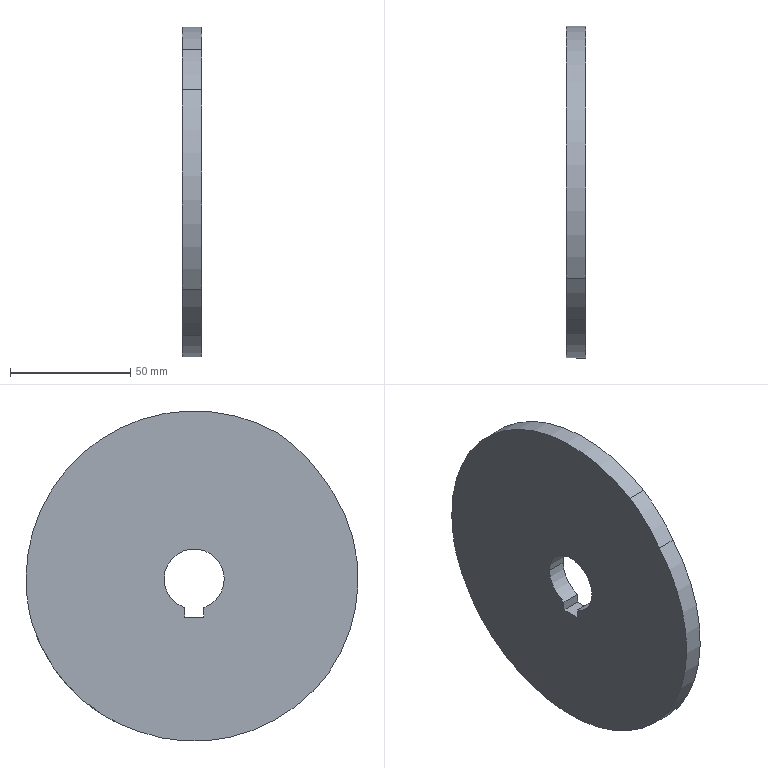Part | NX | 1 solid | 15 faces | box 8 x 138.01 x 137.3 mm | volume 114801 mm3 | cylinder 9 | plane 5 | spline 1 | commonest cylinder face diameters 25 x3 139.8 x2 134.8 x1 135.471 x1 136.22 x1 137.835 x1
STEP:
#1=CARTESIAN_POINT('',(-4.,67.518,-18.091));
#2=VERTEX_POINT('',#1);
#3=CARTESIAN_POINT('',(-4.,69.9,0.));
#4=VERTEX_POINT('',#3);
#5=CARTESIAN_POINT('',(-4.,0.,0.));
#6=DIRECTION('',(1.,0.,0.));
#7=DIRECTION('',(0.,1.,0.));
#8=AXIS2_PLACEMENT_3D('',#5,#6,#7);
#9=CIRCLE('',#8,69.9);
#10=EDGE_CURVE('',#2,#4,#9,.T.);
#11=ORIENTED_EDGE('',*,*,#10,.F.);
#12=CARTESIAN_POINT('',(-4.,23.052,-63.335));
#13=VERTEX_POINT('',#12);
#14=CARTESIAN_POINT('',(-4.,67.518,-18.091));
#15=CARTESIAN_POINT('',(-4.,64.222,-28.782));
#16=CARTESIAN_POINT('',(-4.,52.439,-48.353));
#17=CARTESIAN_POINT('',(-4.,33.356,-60.029));
#18=CARTESIAN_POINT('',(-4.,23.052,-63.335));
#19=B_SPLINE_CURVE_WITH_KNOTS('',3,(#14,#15,#16,#17,#18),.UNSPECIFIED.,.F.,.F.,(4,1,4),(0.,0.5,1.),.UNSPECIFIED.);
#20=EDGE_CURVE('',#13,#2,#19,.F.);
#21=ORIENTED_EDGE('',*,*,#20,.F.);
#22=CARTESIAN_POINT('',(-4.,-33.701,-58.37));
#23=VERTEX_POINT('',#22);
#24=CARTESIAN_POINT('',(-4.,0.,0.));
#25=DIRECTION('',(1.,0.,0.));
#26=DIRECTION('',(0.,-0.5001,-0.866));
#27=AXIS2_PLACEMENT_3D('',#24,#25,#26);
#28=CIRCLE('',#27,67.4);
#29=EDGE_CURVE('',#23,#13,#28,.T.);
#30=ORIENTED_EDGE('',*,*,#29,.F.);
#31=CARTESIAN_POINT('',(-4.,-55.792,-39.066));
#32=VERTEX_POINT('',#31);
#33=CARTESIAN_POINT('',(-4.,-1.234,1.077));
#34=DIRECTION('',(1.,0.,0.));
#35=DIRECTION('',(0.,-0.8055,-0.5926));
#36=AXIS2_PLACEMENT_3D('',#33,#34,#35);
#37=CIRCLE('',#36,67.736);
#38=EDGE_CURVE('',#32,#23,#37,.T.);
#39=ORIENTED_EDGE('',*,*,#38,.F.);
#40=CARTESIAN_POINT('',(-4.,-52.176,43.781));
#41=VERTEX_POINT('',#40);
#42=CARTESIAN_POINT('',(-4.,0.,0.));
#43=DIRECTION('',(1.,0.,0.));
#44=DIRECTION('',(0.,-0.766,0.6428));
#45=AXIS2_PLACEMENT_3D('',#42,#43,#44);
#46=CIRCLE('',#45,68.11);
#47=EDGE_CURVE('',#41,#32,#46,.T.);
#48=ORIENTED_EDGE('',*,*,#47,.F.);
#49=CARTESIAN_POINT('',(-4.,-34.947,60.538));
#50=VERTEX_POINT('',#49);
#51=CARTESIAN_POINT('',(-4.,3.752,3.512));
#52=DIRECTION('',(1.,0.,0.));
#53=DIRECTION('',(0.,-0.5615,0.8275));
#54=AXIS2_PLACEMENT_3D('',#51,#52,#53);
#55=CIRCLE('',#54,68.917);
#56=EDGE_CURVE('',#50,#41,#55,.T.);
#57=ORIENTED_EDGE('',*,*,#56,.F.);
#58=CARTESIAN_POINT('',(-4.,0.,0.));
#59=DIRECTION('',(1.,0.,0.));
#60=DIRECTION('',(0.,1.,0.));
#61=AXIS2_PLACEMENT_3D('',#58,#59,#60);
#62=CIRCLE('',#61,69.9);
#63=EDGE_CURVE('',#4,#50,#62,.T.);
#64=ORIENTED_EDGE('',*,*,#63,.F.);
#65=EDGE_LOOP('',(#11,#21,#30,#39,#48,#57,#64));
#66=FACE_BOUND('',#65,.T.);
#67=CARTESIAN_POINT('',(-4.,-4.,-11.843));
#68=VERTEX_POINT('',#67);
#69=CARTESIAN_POINT('',(-4.,-12.5,0.));
#70=VERTEX_POINT('',#69);
#71=CARTESIAN_POINT('',(-4.,0.,0.));
#72=DIRECTION('',(-1.,0.,0.));
#73=DIRECTION('',(0.,1.,0.));
#74=AXIS2_PLACEMENT_3D('',#71,#72,#73);
#75=CIRCLE('',#74,12.5);
#76=EDGE_CURVE('',#68,#70,#75,.T.);
#77=ORIENTED_EDGE('',*,*,#76,.F.);
#78=CARTESIAN_POINT('',(-4.,-4.,-15.8));
#79=VERTEX_POINT('',#78);
#80=CARTESIAN_POINT('',(-4.,-4.,-11.843));
#81=DIRECTION('',(0.,0.,-1.));
#82=VECTOR('',#81,1000.);
#83=LINE('',#80,#82);
#84=EDGE_CURVE('',#68,#79,#83,.T.);
#85=ORIENTED_EDGE('',*,*,#84,.T.);
#86=CARTESIAN_POINT('',(-4.,4.,-15.8));
#87=VERTEX_POINT('',#86);
#88=CARTESIAN_POINT('',(-4.,-4.,-15.8));
#89=DIRECTION('',(0.,1.,0.));
#90=VECTOR('',#89,1000.);
#91=LINE('',#88,#90);
#92=EDGE_CURVE('',#79,#87,#91,.T.);
#93=ORIENTED_EDGE('',*,*,#92,.T.);
#94=CARTESIAN_POINT('',(-4.,4.,-11.843));
#95=VERTEX_POINT('',#94);
#96=CARTESIAN_POINT('',(-4.,4.,-15.8));
#97=DIRECTION('',(0.,0.,1.));
#98=VECTOR('',#97,1000.);
#99=LINE('',#96,#98);
#100=EDGE_CURVE('',#87,#95,#99,.T.);
#101=ORIENTED_EDGE('',*,*,#100,.T.);
#102=CARTESIAN_POINT('',(-4.,12.5,0.));
#103=VERTEX_POINT('',#102);
#104=CARTESIAN_POINT('',(-4.,0.,0.));
#105=DIRECTION('',(-1.,0.,0.));
#106=DIRECTION('',(0.,1.,0.));
#107=AXIS2_PLACEMENT_3D('',#104,#105,#106);
#108=CIRCLE('',#107,12.5);
#109=EDGE_CURVE('',#103,#95,#108,.T.);
#110=ORIENTED_EDGE('',*,*,#109,.F.);
#111=CARTESIAN_POINT('',(-4.,0.,0.));
#112=DIRECTION('',(-1.,0.,0.));
#113=DIRECTION('',(0.,1.,0.));
#114=AXIS2_PLACEMENT_3D('',#111,#112,#113);
#115=CIRCLE('',#114,12.5);
#116=EDGE_CURVE('',#70,#103,#115,.T.);
#117=ORIENTED_EDGE('',*,*,#116,.F.);
#118=EDGE_LOOP('',(#77,#85,#93,#101,#110,#117));
#119=FACE_BOUND('',#118,.T.);
#120=CARTESIAN_POINT('',(-4.,0.,0.));
#121=DIRECTION('',(1.,0.,0.));
#122=DIRECTION('',(0.,1.,0.));
#123=AXIS2_PLACEMENT_3D('',#120,#121,#122);
#124=PLANE('',#123);
#125=ADVANCED_FACE('',(#66,#119),#124,.F.);
#126=CARTESIAN_POINT('',(4.,69.9,0.));
#127=VERTEX_POINT('',#126);
#128=CARTESIAN_POINT('',(4.,69.9,0.));
#129=DIRECTION('',(-1.,0.,0.));
#130=VECTOR('',#129,1000.);
#131=LINE('',#128,#130);
#132=EDGE_CURVE('',#127,#4,#131,.T.);
#133=ORIENTED_EDGE('',*,*,#132,.F.);
#134=CARTESIAN_POINT('',(4.,67.518,-18.091));
#135=VERTEX_POINT('',#134);
#136=CARTESIAN_POINT('',(4.,0.,0.));
#137=DIRECTION('',(-1.,0.,0.));
#138=DIRECTION('',(0.,-0.4999,0.8661));
#139=AXIS2_PLACEMENT_3D('',#136,#137,#138);
#140=CIRCLE('',#139,69.9);
#141=EDGE_CURVE('',#127,#135,#140,.T.);
#142=ORIENTED_EDGE('',*,*,#141,.T.);
#143=CARTESIAN_POINT('',(4.,67.518,-18.091));
#144=CARTESIAN_POINT('',(1.333,67.518,-18.091));
#145=CARTESIAN_POINT('',(-1.333,67.518,-18.091));
#146=CARTESIAN_POINT('',(-4.,67.518,-18.091));
#147=B_SPLINE_CURVE_WITH_KNOTS('',3,(#143,#144,#145,#146),.UNSPECIFIED.,.F.,.F.,(4,4),(0.,1.),.UNSPECIFIED.);
#148=EDGE_CURVE('',#135,#2,#147,.T.);
#149=ORIENTED_EDGE('',*,*,#148,.T.);
#150=ORIENTED_EDGE('',*,*,#10,.T.);
#151=EDGE_LOOP('',(#133,#142,#149,#150));
#152=FACE_BOUND('',#151,.T.);
#153=CARTESIAN_POINT('',(4.,0.,0.));
#154=DIRECTION('',(-1.,0.,0.));
#155=DIRECTION('',(0.,1.,0.));
#156=AXIS2_PLACEMENT_3D('',#153,#154,#155);
#157=CYLINDRICAL_SURFACE('',#156,69.9);
#158=ADVANCED_FACE('',(#152),#157,.T.);
#159=CARTESIAN_POINT('',(4.,-34.947,60.538));
#160=VERTEX_POINT('',#159);
#161=CARTESIAN_POINT('',(4.,0.,0.));
#162=DIRECTION('',(-1.,0.,0.));
#163=DIRECTION('',(0.,-0.4999,0.8661));
#164=AXIS2_PLACEMENT_3D('',#161,#162,#163);
#165=CIRCLE('',#164,69.9);
#166=EDGE_CURVE('',#160,#127,#165,.T.);
#167=ORIENTED_EDGE('',*,*,#166,.F.);
#168=CARTESIAN_POINT('',(4.,-52.176,43.781));
#169=VERTEX_POINT('',#168);
#170=CARTESIAN_POINT('',(4.,3.752,3.512));
#171=DIRECTION('',(-1.,0.,0.));
#172=DIRECTION('',(0.,-0.8115,0.5843));
#173=AXIS2_PLACEMENT_3D('',#170,#171,#172);
#174=CIRCLE('',#173,68.917);
#175=EDGE_CURVE('',#169,#160,#174,.T.);
#176=ORIENTED_EDGE('',*,*,#175,.F.);
#177=CARTESIAN_POINT('',(4.,-55.792,-39.066));
#178=VERTEX_POINT('',#177);
#179=CARTESIAN_POINT('',(4.,0.,0.));
#180=DIRECTION('',(-1.,0.,0.));
#181=DIRECTION('',(0.,-0.8192,-0.5735));
#182=AXIS2_PLACEMENT_3D('',#179,#180,#181);
#183=CIRCLE('',#182,68.11);
#184=EDGE_CURVE('',#178,#169,#183,.T.);
#185=ORIENTED_EDGE('',*,*,#184,.F.);
#186=CARTESIAN_POINT('',(4.,-33.701,-58.37));
#187=VERTEX_POINT('',#186);
#188=CARTESIAN_POINT('',(4.,-1.234,1.077));
#189=DIRECTION('',(-1.,0.,0.));
#190=DIRECTION('',(0.,-0.4794,-0.8776));
#191=AXIS2_PLACEMENT_3D('',#188,#189,#190);
#192=CIRCLE('',#191,67.736);
#193=EDGE_CURVE('',#187,#178,#192,.T.);
#194=ORIENTED_EDGE('',*,*,#193,.F.);
#195=CARTESIAN_POINT('',(4.,23.052,-63.335));
#196=VERTEX_POINT('',#195);
#197=CARTESIAN_POINT('',(4.,0.,0.));
#198=DIRECTION('',(-1.,0.,0.));
#199=DIRECTION('',(0.,0.342,-0.9397));
#200=AXIS2_PLACEMENT_3D('',#197,#198,#199);
#201=CIRCLE('',#200,67.4);
#202=EDGE_CURVE('',#196,#187,#201,.T.);
#203=ORIENTED_EDGE('',*,*,#202,.F.);
#204=CARTESIAN_POINT('',(4.,23.052,-63.335));
#205=CARTESIAN_POINT('',(4.,33.355,-60.03));
#206=CARTESIAN_POINT('',(4.,52.44,-48.352));
#207=CARTESIAN_POINT('',(4.,64.222,-28.783));
#208=CARTESIAN_POINT('',(4.,67.518,-18.091));
#209=B_SPLINE_CURVE_WITH_KNOTS('',3,(#204,#205,#206,#207,#208),.UNSPECIFIED.,.F.,.F.,(4,1,4),(0.,0.5,1.),.UNSPECIFIED.);
#210=EDGE_CURVE('',#135,#196,#209,.F.);
#211=ORIENTED_EDGE('',*,*,#210,.F.);
#212=ORIENTED_EDGE('',*,*,#141,.F.);
#213=EDGE_LOOP('',(#167,#176,#185,#194,#203,#211,#212));
#214=FACE_BOUND('',#213,.T.);
#215=CARTESIAN_POINT('',(4.,4.,-11.843));
#216=VERTEX_POINT('',#215);
#217=CARTESIAN_POINT('',(4.,12.5,0.));
#218=VERTEX_POINT('',#217);
#219=CARTESIAN_POINT('',(4.,0.,0.));
#220=DIRECTION('',(1.,0.,0.));
#221=DIRECTION('',(0.,-1.,0.));
#222=AXIS2_PLACEMENT_3D('',#219,#220,#221);
#223=CIRCLE('',#222,12.5);
#224=EDGE_CURVE('',#216,#218,#223,.T.);
#225=ORIENTED_EDGE('',*,*,#224,.F.);
#226=CARTESIAN_POINT('',(4.,4.,-15.8));
#227=VERTEX_POINT('',#226);
#228=CARTESIAN_POINT('',(4.,4.,-15.8));
#229=DIRECTION('',(0.,0.,1.));
#230=VECTOR('',#229,1000.);
#231=LINE('',#228,#230);
#232=EDGE_CURVE('',#227,#216,#231,.T.);
#233=ORIENTED_EDGE('',*,*,#232,.F.);
#234=CARTESIAN_POINT('',(4.,-4.,-15.8));
#235=VERTEX_POINT('',#234);
#236=CARTESIAN_POINT('',(4.,-4.,-15.8));
#237=DIRECTION('',(0.,1.,0.));
#238=VECTOR('',#237,1000.);
#239=LINE('',#236,#238);
#240=EDGE_CURVE('',#235,#227,#239,.T.);
#241=ORIENTED_EDGE('',*,*,#240,.F.);
#242=CARTESIAN_POINT('',(4.,-4.,-11.843));
#243=VERTEX_POINT('',#242);
#244=CARTESIAN_POINT('',(4.,-4.,-11.843));
#245=DIRECTION('',(0.,0.,-1.));
#246=VECTOR('',#245,1000.);
#247=LINE('',#244,#246);
#248=EDGE_CURVE('',#243,#235,#247,.T.);
#249=ORIENTED_EDGE('',*,*,#248,.F.);
#250=CARTESIAN_POINT('',(4.,-12.5,0.));
#251=VERTEX_POINT('',#250);
#252=CARTESIAN_POINT('',(4.,0.,0.));
#253=DIRECTION('',(1.,0.,0.));
#254=DIRECTION('',(0.,-1.,0.));
#255=AXIS2_PLACEMENT_3D('',#252,#253,#254);
#256=CIRCLE('',#255,12.5);
#257=EDGE_CURVE('',#251,#243,#256,.T.);
#258=ORIENTED_EDGE('',*,*,#257,.F.);
#259=CARTESIAN_POINT('',(4.,0.,0.));
#260=DIRECTION('',(1.,0.,0.));
#261=DIRECTION('',(0.,-1.,0.));
#262=AXIS2_PLACEMENT_3D('',#259,#260,#261);
#263=CIRCLE('',#262,12.5);
#264=EDGE_CURVE('',#218,#251,#263,.T.);
#265=ORIENTED_EDGE('',*,*,#264,.F.);
#266=EDGE_LOOP('',(#225,#233,#241,#249,#258,#265));
#267=FACE_BOUND('',#266,.T.);
#268=CARTESIAN_POINT('',(4.,0.,0.));
#269=DIRECTION('',(1.,0.,0.));
#270=DIRECTION('',(0.,1.,0.));
#271=AXIS2_PLACEMENT_3D('',#268,#269,#270);
#272=PLANE('',#271);
#273=ADVANCED_FACE('',(#214,#267),#272,.T.);
#274=ORIENTED_EDGE('',*,*,#20,.T.);
#275=ORIENTED_EDGE('',*,*,#148,.F.);
#276=ORIENTED_EDGE('',*,*,#210,.T.);
#277=CARTESIAN_POINT('',(-4.,23.052,-63.335));
#278=CARTESIAN_POINT('',(-1.333,23.052,-63.335));
#279=CARTESIAN_POINT('',(1.333,23.052,-63.335));
#280=CARTESIAN_POINT('',(4.,23.052,-63.335));
#281=B_SPLINE_CURVE_WITH_KNOTS('',3,(#277,#278,#279,#280),.UNSPECIFIED.,.F.,.F.,(4,4),(0.,1.),.UNSPECIFIED.);
#282=EDGE_CURVE('',#196,#13,#281,.F.);
#283=ORIENTED_EDGE('',*,*,#282,.T.);
#284=EDGE_LOOP('',(#274,#275,#276,#283));
#285=FACE_BOUND('',#284,.T.);
#286=CARTESIAN_POINT('',(4.,67.518,-18.091));
#287=CARTESIAN_POINT('',(-4.,67.518,-18.091));
#288=CARTESIAN_POINT('',(4.,64.221,-28.786));
#289=CARTESIAN_POINT('',(-4.,64.221,-28.786));
#290=CARTESIAN_POINT('',(4.,52.454,-48.346));
#291=CARTESIAN_POINT('',(-4.,52.454,-48.346));
#292=CARTESIAN_POINT('',(4.,33.328,-60.038));
#293=CARTESIAN_POINT('',(-4.,33.328,-60.038));
#294=CARTESIAN_POINT('',(4.,23.052,-63.335));
#295=CARTESIAN_POINT('',(-4.,23.052,-63.335));
#296=B_SPLINE_SURFACE_WITH_KNOTS('',3,1,((#286,#287),(#288,#289),(#290,#291),(#292,#293),(#294,#295)),.SURF_OF_LINEAR_EXTRUSION.,.F.,.F.,.F.,(4,1,4),(2,2),(0.009627,0.4998,0.99),(0.,1.),.UNSPECIFIED.);
#297=ADVANCED_FACE('',(#285),#296,.T.);
#298=ORIENTED_EDGE('',*,*,#29,.T.);
#299=ORIENTED_EDGE('',*,*,#282,.F.);
#300=ORIENTED_EDGE('',*,*,#202,.T.);
#301=CARTESIAN_POINT('',(4.,-33.701,-58.37));
#302=CARTESIAN_POINT('',(1.333,-33.701,-58.37));
#303=CARTESIAN_POINT('',(-1.333,-33.701,-58.37));
#304=CARTESIAN_POINT('',(-4.,-33.701,-58.37));
#305=B_SPLINE_CURVE_WITH_KNOTS('',3,(#301,#302,#303,#304),.UNSPECIFIED.,.F.,.F.,(4,4),(0.,1.),.UNSPECIFIED.);
#306=EDGE_CURVE('',#187,#23,#305,.T.);
#307=ORIENTED_EDGE('',*,*,#306,.T.);
#308=EDGE_LOOP('',(#298,#299,#300,#307));
#309=FACE_BOUND('',#308,.T.);
#310=CARTESIAN_POINT('',(4.,0.,0.));
#311=DIRECTION('',(-1.,0.,0.));
#312=DIRECTION('',(0.,0.342,-0.9397));
#313=AXIS2_PLACEMENT_3D('',#310,#311,#312);
#314=CYLINDRICAL_SURFACE('',#313,67.4);
#315=ADVANCED_FACE('',(#309),#314,.T.);
#316=ORIENTED_EDGE('',*,*,#38,.T.);
#317=ORIENTED_EDGE('',*,*,#306,.F.);
#318=ORIENTED_EDGE('',*,*,#193,.T.);
#319=CARTESIAN_POINT('',(4.,-55.792,-39.066));
#320=CARTESIAN_POINT('',(1.333,-55.792,-39.066));
#321=CARTESIAN_POINT('',(-1.333,-55.792,-39.066));
#322=CARTESIAN_POINT('',(-4.,-55.792,-39.066));
#323=B_SPLINE_CURVE_WITH_KNOTS('',3,(#319,#320,#321,#322),.UNSPECIFIED.,.F.,.F.,(4,4),(0.,1.),.UNSPECIFIED.);
#324=EDGE_CURVE('',#178,#32,#323,.T.);
#325=ORIENTED_EDGE('',*,*,#324,.T.);
#326=EDGE_LOOP('',(#316,#317,#318,#325));
#327=FACE_BOUND('',#326,.T.);
#328=CARTESIAN_POINT('',(0.,-1.234,1.077));
#329=DIRECTION('',(-1.,0.,0.));
#330=DIRECTION('',(0.,-0.4793,-0.8776));
#331=AXIS2_PLACEMENT_3D('',#328,#329,#330);
#332=CYLINDRICAL_SURFACE('',#331,67.736);
#333=ADVANCED_FACE('',(#327),#332,.T.);
#334=ORIENTED_EDGE('',*,*,#47,.T.);
#335=ORIENTED_EDGE('',*,*,#324,.F.);
#336=ORIENTED_EDGE('',*,*,#184,.T.);
#337=CARTESIAN_POINT('',(4.,-52.175,43.78));
#338=CARTESIAN_POINT('',(1.333,-52.175,43.78));
#339=CARTESIAN_POINT('',(-1.333,-52.175,43.78));
#340=CARTESIAN_POINT('',(-4.,-52.175,43.78));
#341=B_SPLINE_CURVE_WITH_KNOTS('',3,(#337,#338,#339,#340),.UNSPECIFIED.,.F.,.F.,(4,4),(0.,1.),.UNSPECIFIED.);
#342=EDGE_CURVE('',#169,#41,#341,.T.);
#343=ORIENTED_EDGE('',*,*,#342,.T.);
#344=EDGE_LOOP('',(#334,#335,#336,#343));
#345=FACE_BOUND('',#344,.T.);
#346=CARTESIAN_POINT('',(4.,0.,0.));
#347=DIRECTION('',(-1.,0.,0.));
#348=DIRECTION('',(0.,-0.8192,-0.5736));
#349=AXIS2_PLACEMENT_3D('',#346,#347,#348);
#350=CYLINDRICAL_SURFACE('',#349,68.11);
#351=ADVANCED_FACE('',(#345),#350,.T.);
#352=ORIENTED_EDGE('',*,*,#56,.T.);
#353=ORIENTED_EDGE('',*,*,#342,.F.);
#354=ORIENTED_EDGE('',*,*,#175,.T.);
#355=CARTESIAN_POINT('',(4.,-34.947,60.538));
#356=CARTESIAN_POINT('',(1.336,-34.949,60.537));
#357=CARTESIAN_POINT('',(-1.331,-34.949,60.537));
#358=CARTESIAN_POINT('',(-4.,-34.947,60.538));
#359=B_SPLINE_CURVE_WITH_KNOTS('',3,(#355,#356,#357,#358),.UNSPECIFIED.,.F.,.F.,(4,4),(0.,1.),.UNSPECIFIED.);
#360=EDGE_CURVE('',#50,#160,#359,.F.);
#361=ORIENTED_EDGE('',*,*,#360,.F.);
#362=EDGE_LOOP('',(#352,#353,#354,#361));
#363=FACE_BOUND('',#362,.T.);
#364=CARTESIAN_POINT('',(0.,3.752,3.512));
#365=DIRECTION('',(-1.,0.,0.));
#366=DIRECTION('',(0.,-0.8115,0.5843));
#367=AXIS2_PLACEMENT_3D('',#364,#365,#366);
#368=CYLINDRICAL_SURFACE('',#367,68.917);
#369=ADVANCED_FACE('',(#363),#368,.T.);
#370=CARTESIAN_POINT('',(-4.4,12.5,0.));
#371=DIRECTION('',(1.,0.,0.));
#372=VECTOR('',#371,1000.);
#373=LINE('',#370,#372);
#374=EDGE_CURVE('',#103,#218,#373,.T.);
#375=ORIENTED_EDGE('',*,*,#374,.F.);
#376=ORIENTED_EDGE('',*,*,#109,.T.);
#377=CARTESIAN_POINT('',(4.,4.,-11.843));
#378=DIRECTION('',(-1.,0.,0.));
#379=VECTOR('',#378,1000.);
#380=LINE('',#377,#379);
#381=EDGE_CURVE('',#216,#95,#380,.T.);
#382=ORIENTED_EDGE('',*,*,#381,.F.);
#383=ORIENTED_EDGE('',*,*,#224,.T.);
#384=EDGE_LOOP('',(#375,#376,#382,#383));
#385=FACE_BOUND('',#384,.T.);
#386=CARTESIAN_POINT('',(-4.4,0.,0.));
#387=DIRECTION('',(1.,0.,0.));
#388=DIRECTION('',(0.,-1.,0.));
#389=AXIS2_PLACEMENT_3D('',#386,#387,#388);
#390=CYLINDRICAL_SURFACE('',#389,12.5);
#391=ADVANCED_FACE('',(#385),#390,.F.);
#392=ORIENTED_EDGE('',*,*,#84,.F.);
#393=CARTESIAN_POINT('',(-4.,-4.,-11.843));
#394=DIRECTION('',(1.,0.,0.));
#395=VECTOR('',#394,1000.);
#396=LINE('',#393,#395);
#397=EDGE_CURVE('',#68,#243,#396,.T.);
#398=ORIENTED_EDGE('',*,*,#397,.T.);
#399=ORIENTED_EDGE('',*,*,#248,.T.);
#400=CARTESIAN_POINT('',(4.,-4.,-15.8));
#401=DIRECTION('',(-1.,0.,0.));
#402=VECTOR('',#401,1000.);
#403=LINE('',#400,#402);
#404=EDGE_CURVE('',#235,#79,#403,.T.);
#405=ORIENTED_EDGE('',*,*,#404,.T.);
#406=EDGE_LOOP('',(#392,#398,#399,#405));
#407=FACE_BOUND('',#406,.T.);
#408=CARTESIAN_POINT('',(-4.,-4.,-15.8));
#409=DIRECTION('',(0.,-1.,0.));
#410=DIRECTION('',(0.,0.,-1.));
#411=AXIS2_PLACEMENT_3D('',#408,#409,#410);
#412=PLANE('',#411);
#413=ADVANCED_FACE('',(#407),#412,.F.);
#414=ORIENTED_EDGE('',*,*,#92,.F.);
#415=ORIENTED_EDGE('',*,*,#404,.F.);
#416=ORIENTED_EDGE('',*,*,#240,.T.);
#417=CARTESIAN_POINT('',(4.,4.,-15.8));
#418=DIRECTION('',(-1.,0.,0.));
#419=VECTOR('',#418,1000.);
#420=LINE('',#417,#419);
#421=EDGE_CURVE('',#227,#87,#420,.T.);
#422=ORIENTED_EDGE('',*,*,#421,.T.);
#423=EDGE_LOOP('',(#414,#415,#416,#422));
#424=FACE_BOUND('',#423,.T.);
#425=CARTESIAN_POINT('',(-4.,4.,-15.8));
#426=DIRECTION('',(0.,0.,-1.));
#427=DIRECTION('',(0.,-1.,0.));
#428=AXIS2_PLACEMENT_3D('',#425,#426,#427);
#429=PLANE('',#428);
#430=ADVANCED_FACE('',(#424),#429,.F.);
#431=ORIENTED_EDGE('',*,*,#100,.F.);
#432=ORIENTED_EDGE('',*,*,#421,.F.);
#433=ORIENTED_EDGE('',*,*,#232,.T.);
#434=ORIENTED_EDGE('',*,*,#381,.T.);
#435=EDGE_LOOP('',(#431,#432,#433,#434));
#436=FACE_BOUND('',#435,.T.);
#437=CARTESIAN_POINT('',(-4.,4.,-11.843));
#438=DIRECTION('',(0.,1.,0.));
#439=DIRECTION('',(1.,0.,0.));
#440=AXIS2_PLACEMENT_3D('',#437,#438,#439);
#441=PLANE('',#440);
#442=ADVANCED_FACE('',(#436),#441,.F.);
#443=ORIENTED_EDGE('',*,*,#76,.T.);
#444=CARTESIAN_POINT('',(-4.4,-12.5,0.));
#445=DIRECTION('',(1.,0.,0.));
#446=VECTOR('',#445,1000.);
#447=LINE('',#444,#446);
#448=EDGE_CURVE('',#70,#251,#447,.T.);
#449=ORIENTED_EDGE('',*,*,#448,.T.);
#450=ORIENTED_EDGE('',*,*,#257,.T.);
#451=ORIENTED_EDGE('',*,*,#397,.F.);
#452=EDGE_LOOP('',(#443,#449,#450,#451));
#453=FACE_BOUND('',#452,.T.);
#454=CARTESIAN_POINT('',(-4.4,0.,0.));
#455=DIRECTION('',(1.,0.,0.));
#456=DIRECTION('',(0.,-1.,0.));
#457=AXIS2_PLACEMENT_3D('',#454,#455,#456);
#458=CYLINDRICAL_SURFACE('',#457,12.5);
#459=ADVANCED_FACE('',(#453),#458,.F.);
#460=ORIENTED_EDGE('',*,*,#116,.T.);
#461=ORIENTED_EDGE('',*,*,#374,.T.);
#462=ORIENTED_EDGE('',*,*,#264,.T.);
#463=ORIENTED_EDGE('',*,*,#448,.F.);
#464=EDGE_LOOP('',(#460,#461,#462,#463));
#465=FACE_BOUND('',#464,.T.);
#466=CARTESIAN_POINT('',(-4.4,0.,0.));
#467=DIRECTION('',(1.,0.,0.));
#468=DIRECTION('',(0.,-1.,0.));
#469=AXIS2_PLACEMENT_3D('',#466,#467,#468);
#470=CYLINDRICAL_SURFACE('',#469,12.5);
#471=ADVANCED_FACE('',(#465),#470,.F.);
#472=ORIENTED_EDGE('',*,*,#166,.T.);
#473=ORIENTED_EDGE('',*,*,#132,.T.);
#474=ORIENTED_EDGE('',*,*,#63,.T.);
#475=ORIENTED_EDGE('',*,*,#360,.T.);
#476=EDGE_LOOP('',(#472,#473,#474,#475));
#477=FACE_BOUND('',#476,.T.);
#478=CARTESIAN_POINT('',(4.,0.,0.));
#479=DIRECTION('',(-1.,0.,0.));
#480=DIRECTION('',(0.,1.,0.));
#481=AXIS2_PLACEMENT_3D('',#478,#479,#480);
#482=CYLINDRICAL_SURFACE('',#481,69.9);
#483=ADVANCED_FACE('',(#477),#482,.T.);
#484=CLOSED_SHELL('',(#125,#158,#273,#297,#315,#333,#351,#369,#391,#413,#430,#442,#459,#471,#483));
#485=MANIFOLD_SOLID_BREP('',#484);
#486=(LENGTH_UNIT()NAMED_UNIT(*)SI_UNIT(.MILLI.,.METRE.));
#487=UNCERTAINTY_MEASURE_WITH_UNIT(LENGTH_MEASURE(0.0508),#486,'','');
#488=(NAMED_UNIT(*)PLANE_ANGLE_UNIT()SI_UNIT($,.RADIAN.));
#489=(NAMED_UNIT(*)SI_UNIT($,.STERADIAN.)SOLID_ANGLE_UNIT());
#490=(GEOMETRIC_REPRESENTATION_CONTEXT(3)GLOBAL_UNCERTAINTY_ASSIGNED_CONTEXT((#487))GLOBAL_UNIT_ASSIGNED_CONTEXT((#486,#488,#489))REPRESENTATION_CONTEXT('',''));
#491=ADVANCED_BREP_SHAPE_REPRESENTATION('',(#485),#490);